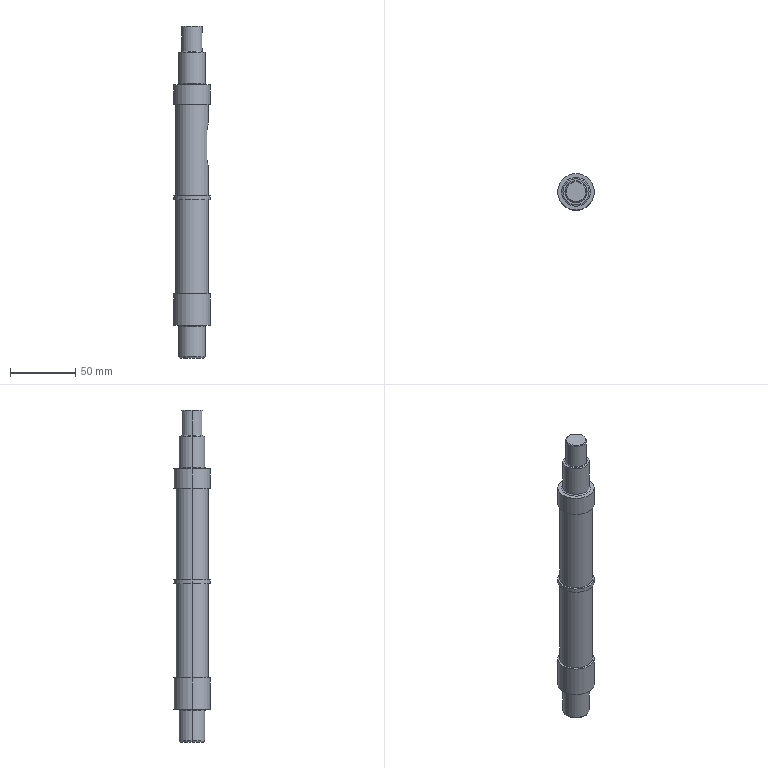Part | SolidWorks | features ICE 6, Fillet 3, Chamfer 2, Revolution 1 | 1 solid | 47 faces | box 28 x 28 x 254.001 mm | volume 113711 mm3 | cylinder 21 | plane 14 | torus 6 | cone 4 | spline 2 | commonest cylinder face diameters 28 x6 16 x4 20 x4 25 x4 10 x3
STEP:
#1=CARTESIAN_POINT('',(7.5,0.,-107.));
#2=VERTEX_POINT('',#1);
#3=CARTESIAN_POINT('',(7.5,5.,-102.));
#4=VERTEX_POINT('',#3);
#5=CARTESIAN_POINT('',(7.5,0.,-102.));
#6=DIRECTION('',(1.,0.,0.));
#7=DIRECTION('',(0.,0.,-1.));
#8=AXIS2_PLACEMENT_3D('',#5,#6,#7);
#9=CIRCLE('',#8,5.);
#10=EDGE_CURVE('',#2,#4,#9,.T.);
#11=ORIENTED_EDGE('',*,*,#10,.F.);
#12=CARTESIAN_POINT('',(12.5,0.,-107.));
#13=VERTEX_POINT('',#12);
#14=CARTESIAN_POINT('',(7.5,0.,-107.));
#15=DIRECTION('',(1.,0.,0.));
#16=VECTOR('',#15,1000.);
#17=LINE('',#14,#16);
#18=EDGE_CURVE('',#2,#13,#17,.T.);
#19=ORIENTED_EDGE('',*,*,#18,.T.);
#20=CARTESIAN_POINT('',(11.456,5.,-102.));
#21=VERTEX_POINT('',#20);
#22=CARTESIAN_POINT('',(11.456,5.,-102.));
#23=CARTESIAN_POINT('',(11.456,5.,-102.334));
#24=CARTESIAN_POINT('',(11.471,4.967,-102.662));
#25=CARTESIAN_POINT('',(11.526,4.838,-103.306));
#26=CARTESIAN_POINT('',(11.567,4.74,-103.625));
#27=CARTESIAN_POINT('',(11.667,4.488,-104.229));
#28=CARTESIAN_POINT('',(11.726,4.334,-104.515));
#29=CARTESIAN_POINT('',(11.854,3.971,-105.056));
#30=CARTESIAN_POINT('',(11.923,3.763,-105.309));
#31=CARTESIAN_POINT('',(12.057,3.306,-105.765));
#32=CARTESIAN_POINT('',(12.124,3.055,-105.971));
#33=CARTESIAN_POINT('',(12.248,2.511,-106.336));
#34=CARTESIAN_POINT('',(12.304,2.225,-106.489));
#35=CARTESIAN_POINT('',(12.374,1.774,-106.677));
#36=CARTESIAN_POINT('',(12.396,1.621,-106.733));
#37=CARTESIAN_POINT('',(12.433,1.305,-106.829));
#38=CARTESIAN_POINT('',(12.449,1.143,-106.87));
#39=CARTESIAN_POINT('',(12.487,0.6575,-106.968));
#40=CARTESIAN_POINT('',(12.5,0.3304,-107.));
#41=CARTESIAN_POINT('',(12.5,0.,-107.));
#42=B_SPLINE_CURVE_WITH_KNOTS('',3,(#22,#23,#24,#25,#26,#27,#28,#29,#30,#31,#32,#33,#34,#35,#36,#37,#38,#39,#40,#41),.UNSPECIFIED.,.F.,.F.,(4,2,2,2,2,2,2,2,2,4),(0.,0.0009877,0.001975,0.002963,0.003951,0.004939,0.005926,0.00642,0.006914,0.007902),.UNSPECIFIED.);
#43=EDGE_CURVE('',#21,#13,#42,.T.);
#44=ORIENTED_EDGE('',*,*,#43,.F.);
#45=CARTESIAN_POINT('',(7.5,5.,-102.));
#46=DIRECTION('',(1.,0.,0.));
#47=VECTOR('',#46,1000.);
#48=LINE('',#45,#47);
#49=EDGE_CURVE('',#4,#21,#48,.T.);
#50=ORIENTED_EDGE('',*,*,#49,.F.);
#51=EDGE_LOOP('',(#11,#19,#44,#50));
#52=FACE_OUTER_BOUND('',#51,.T.);
#53=CARTESIAN_POINT('',(7.5,0.,-102.));
#54=DIRECTION('',(1.,0.,0.));
#55=DIRECTION('',(0.,0.,-1.));
#56=AXIS2_PLACEMENT_3D('',#53,#54,#55);
#57=CYLINDRICAL_SURFACE('',#56,5.);
#58=ADVANCED_FACE('',(#52),#57,.F.);
#59=CARTESIAN_POINT('',(-12.5,0.,-130.));
#60=VERTEX_POINT('',#59);
#61=CARTESIAN_POINT('',(12.5,0.,-130.));
#62=VERTEX_POINT('',#61);
#63=CARTESIAN_POINT('',(0.,0.,-130.));
#64=DIRECTION('',(0.,0.,-1.));
#65=DIRECTION('',(-1.,0.,0.));
#66=AXIS2_PLACEMENT_3D('',#63,#64,#65);
#67=CIRCLE('',#66,12.5);
#68=EDGE_CURVE('',#60,#62,#67,.T.);
#69=ORIENTED_EDGE('',*,*,#68,.F.);
#70=CARTESIAN_POINT('',(-12.5,0.,-60.));
#71=VERTEX_POINT('',#70);
#72=CARTESIAN_POINT('',(-12.5,0.,0.));
#73=DIRECTION('',(0.,0.,1.));
#74=VECTOR('',#73,1000.);
#75=LINE('',#72,#74);
#76=EDGE_CURVE('',#60,#71,#75,.T.);
#77=ORIENTED_EDGE('',*,*,#76,.T.);
#78=CARTESIAN_POINT('',(12.5,0.,-60.));
#79=VERTEX_POINT('',#78);
#80=CARTESIAN_POINT('',(0.,0.,-60.));
#81=DIRECTION('',(0.,0.,1.));
#82=DIRECTION('',(1.,0.,0.));
#83=AXIS2_PLACEMENT_3D('',#80,#81,#82);
#84=CIRCLE('',#83,12.5);
#85=EDGE_CURVE('',#79,#71,#84,.T.);
#86=ORIENTED_EDGE('',*,*,#85,.F.);
#87=CARTESIAN_POINT('',(12.5,0.,-75.));
#88=VERTEX_POINT('',#87);
#89=CARTESIAN_POINT('',(12.5,0.,0.));
#90=DIRECTION('',(0.,0.,1.));
#91=VECTOR('',#90,1000.);
#92=LINE('',#89,#91);
#93=EDGE_CURVE('',#88,#79,#92,.T.);
#94=ORIENTED_EDGE('',*,*,#93,.F.);
#95=CARTESIAN_POINT('',(11.456,5.,-80.));
#96=VERTEX_POINT('',#95);
#97=CARTESIAN_POINT('',(12.5,0.,-75.));
#98=CARTESIAN_POINT('',(12.5,0.3299,-75.));
#99=CARTESIAN_POINT('',(12.487,0.6645,-75.033));
#100=CARTESIAN_POINT('',(12.436,1.308,-75.163));
#101=CARTESIAN_POINT('',(12.398,1.622,-75.259));
#102=CARTESIAN_POINT('',(12.303,2.231,-75.513));
#103=CARTESIAN_POINT('',(12.247,2.517,-75.668));
#104=CARTESIAN_POINT('',(12.124,3.055,-76.029));
#105=CARTESIAN_POINT('',(12.056,3.309,-76.238));
#106=CARTESIAN_POINT('',(11.922,3.766,-76.695));
#107=CARTESIAN_POINT('',(11.854,3.97,-76.944));
#108=CARTESIAN_POINT('',(11.727,4.332,-77.483));
#109=CARTESIAN_POINT('',(11.667,4.489,-77.773));
#110=CARTESIAN_POINT('',(11.568,4.739,-78.373));
#111=CARTESIAN_POINT('',(11.527,4.835,-78.684));
#112=CARTESIAN_POINT('',(11.471,4.967,-79.334));
#113=CARTESIAN_POINT('',(11.456,5.,-79.666));
#114=CARTESIAN_POINT('',(11.456,5.,-80.));
#115=B_SPLINE_CURVE_WITH_KNOTS('',3,(#97,#98,#99,#100,#101,#102,#103,#104,#105,#106,#107,#108,#109,#110,#111,#112,#113,#114),.UNSPECIFIED.,.F.,.F.,(4,2,2,2,2,2,2,2,4),(0.007902,0.008888,0.009874,0.01086,0.01185,0.01283,0.01382,0.01481,0.01579),.UNSPECIFIED.);
#116=EDGE_CURVE('',#88,#96,#115,.T.);
#117=ORIENTED_EDGE('',*,*,#116,.T.);
#118=CARTESIAN_POINT('',(11.456,5.,0.));
#119=DIRECTION('',(0.,0.,-1.));
#120=VECTOR('',#119,1000.);
#121=LINE('',#118,#120);
#122=EDGE_CURVE('',#96,#21,#121,.T.);
#123=ORIENTED_EDGE('',*,*,#122,.T.);
#124=ORIENTED_EDGE('',*,*,#43,.T.);
#125=CARTESIAN_POINT('',(12.5,0.,0.));
#126=DIRECTION('',(0.,0.,1.));
#127=VECTOR('',#126,1000.);
#128=LINE('',#125,#127);
#129=EDGE_CURVE('',#62,#13,#128,.T.);
#130=ORIENTED_EDGE('',*,*,#129,.F.);
#131=EDGE_LOOP('',(#69,#77,#86,#94,#117,#123,#124,#130));
#132=FACE_OUTER_BOUND('',#131,.T.);
#133=CARTESIAN_POINT('',(0.,0.,0.));
#134=DIRECTION('',(0.,0.,1.));
#135=DIRECTION('',(1.,0.,0.));
#136=AXIS2_PLACEMENT_3D('',#133,#134,#135);
#137=CYLINDRICAL_SURFACE('',#136,12.5);
#138=ADVANCED_FACE('',(#132),#137,.T.);
#139=CARTESIAN_POINT('',(14.,0.,-60.));
#140=VERTEX_POINT('',#139);
#141=CARTESIAN_POINT('',(-14.,0.,-60.));
#142=VERTEX_POINT('',#141);
#143=CARTESIAN_POINT('',(0.,0.,-60.));
#144=DIRECTION('',(0.,0.,1.));
#145=DIRECTION('',(1.,0.,0.));
#146=AXIS2_PLACEMENT_3D('',#143,#144,#145);
#147=CIRCLE('',#146,14.);
#148=EDGE_CURVE('',#140,#142,#147,.T.);
#149=ORIENTED_EDGE('',*,*,#148,.T.);
#150=CARTESIAN_POINT('',(-14.,0.,-45.));
#151=VERTEX_POINT('',#150);
#152=CARTESIAN_POINT('',(-14.,0.,0.));
#153=DIRECTION('',(0.,0.,1.));
#154=VECTOR('',#153,1000.);
#155=LINE('',#152,#154);
#156=EDGE_CURVE('',#142,#151,#155,.T.);
#157=ORIENTED_EDGE('',*,*,#156,.T.);
#158=CARTESIAN_POINT('',(14.,0.,-45.));
#159=VERTEX_POINT('',#158);
#160=CARTESIAN_POINT('',(0.,0.,-45.));
#161=DIRECTION('',(0.,0.,1.));
#162=DIRECTION('',(1.,0.,0.));
#163=AXIS2_PLACEMENT_3D('',#160,#161,#162);
#164=CIRCLE('',#163,14.);
#165=EDGE_CURVE('',#159,#151,#164,.T.);
#166=ORIENTED_EDGE('',*,*,#165,.F.);
#167=CARTESIAN_POINT('',(14.,0.,0.));
#168=DIRECTION('',(0.,0.,1.));
#169=VECTOR('',#168,1000.);
#170=LINE('',#167,#169);
#171=EDGE_CURVE('',#140,#159,#170,.T.);
#172=ORIENTED_EDGE('',*,*,#171,.F.);
#173=EDGE_LOOP('',(#149,#157,#166,#172));
#174=FACE_OUTER_BOUND('',#173,.T.);
#175=CARTESIAN_POINT('',(0.,0.,0.));
#176=DIRECTION('',(0.,0.,1.));
#177=DIRECTION('',(1.,0.,0.));
#178=AXIS2_PLACEMENT_3D('',#175,#176,#177);
#179=CYLINDRICAL_SURFACE('',#178,14.);
#180=ADVANCED_FACE('',(#174),#179,.T.);
#181=CARTESIAN_POINT('',(11.,0.,-45.));
#182=VERTEX_POINT('',#181);
#183=CARTESIAN_POINT('',(-11.,0.,-45.));
#184=VERTEX_POINT('',#183);
#185=CARTESIAN_POINT('',(0.,0.,-45.));
#186=DIRECTION('',(0.,0.,-1.));
#187=DIRECTION('',(-1.,0.,0.));
#188=AXIS2_PLACEMENT_3D('',#185,#186,#187);
#189=CIRCLE('',#188,11.);
#190=EDGE_CURVE('',#182,#184,#189,.T.);
#191=ORIENTED_EDGE('',*,*,#190,.F.);
#192=CARTESIAN_POINT('',(10.,0.,-44.));
#193=VERTEX_POINT('',#192);
#194=CARTESIAN_POINT('',(11.,0.,-44.));
#195=DIRECTION('',(0.,1.,0.));
#196=DIRECTION('',(-1.,0.,0.));
#197=AXIS2_PLACEMENT_3D('',#194,#195,#196);
#198=CIRCLE('',#197,1.);
#199=EDGE_CURVE('',#182,#193,#198,.T.);
#200=ORIENTED_EDGE('',*,*,#199,.T.);
#201=CARTESIAN_POINT('',(-10.,0.,-44.));
#202=VERTEX_POINT('',#201);
#203=CARTESIAN_POINT('',(0.,0.,-44.));
#204=DIRECTION('',(0.,0.,1.));
#205=DIRECTION('',(-1.,0.,0.));
#206=AXIS2_PLACEMENT_3D('',#203,#204,#205);
#207=CIRCLE('',#206,10.);
#208=EDGE_CURVE('',#202,#193,#207,.T.);
#209=ORIENTED_EDGE('',*,*,#208,.F.);
#210=CARTESIAN_POINT('',(-11.,0.,-44.));
#211=DIRECTION('',(0.,-1.,0.));
#212=DIRECTION('',(0.,0.,-1.));
#213=AXIS2_PLACEMENT_3D('',#210,#211,#212);
#214=CIRCLE('',#213,1.);
#215=EDGE_CURVE('',#184,#202,#214,.T.);
#216=ORIENTED_EDGE('',*,*,#215,.F.);
#217=EDGE_LOOP('',(#191,#200,#209,#216));
#218=FACE_OUTER_BOUND('',#217,.T.);
#219=CARTESIAN_POINT('',(0.,0.,-44.));
#220=DIRECTION('',(0.,0.,-1.));
#221=DIRECTION('',(-1.,0.,0.));
#222=AXIS2_PLACEMENT_3D('',#219,#220,#221);
#223=TOROIDAL_SURFACE('',#222,11.,1.);
#224=ADVANCED_FACE('',(#218),#223,.F.);
#225=CARTESIAN_POINT('',(0.,0.,-44.));
#226=DIRECTION('',(0.,0.,1.));
#227=DIRECTION('',(-1.,0.,0.));
#228=AXIS2_PLACEMENT_3D('',#225,#226,#227);
#229=CIRCLE('',#228,10.);
#230=EDGE_CURVE('',#193,#202,#229,.T.);
#231=ORIENTED_EDGE('',*,*,#230,.T.);
#232=CARTESIAN_POINT('',(-10.,0.,-20.));
#233=VERTEX_POINT('',#232);
#234=CARTESIAN_POINT('',(-10.,0.,0.));
#235=DIRECTION('',(0.,0.,1.));
#236=VECTOR('',#235,1000.);
#237=LINE('',#234,#236);
#238=EDGE_CURVE('',#202,#233,#237,.T.);
#239=ORIENTED_EDGE('',*,*,#238,.T.);
#240=CARTESIAN_POINT('',(10.,0.,-20.));
#241=VERTEX_POINT('',#240);
#242=CARTESIAN_POINT('',(0.,0.,-20.));
#243=DIRECTION('',(0.,0.,1.));
#244=DIRECTION('',(1.,0.,0.));
#245=AXIS2_PLACEMENT_3D('',#242,#243,#244);
#246=CIRCLE('',#245,10.);
#247=EDGE_CURVE('',#241,#233,#246,.T.);
#248=ORIENTED_EDGE('',*,*,#247,.F.);
#249=CARTESIAN_POINT('',(10.,0.,0.));
#250=DIRECTION('',(0.,0.,1.));
#251=VECTOR('',#250,1000.);
#252=LINE('',#249,#251);
#253=EDGE_CURVE('',#193,#241,#252,.T.);
#254=ORIENTED_EDGE('',*,*,#253,.F.);
#255=EDGE_LOOP('',(#231,#239,#248,#254));
#256=FACE_OUTER_BOUND('',#255,.T.);
#257=CARTESIAN_POINT('',(0.,0.,0.));
#258=DIRECTION('',(0.,0.,1.));
#259=DIRECTION('',(1.,0.,0.));
#260=AXIS2_PLACEMENT_3D('',#257,#258,#259);
#261=CYLINDRICAL_SURFACE('',#260,10.);
#262=ADVANCED_FACE('',(#256),#261,.T.);
#263=CARTESIAN_POINT('',(8.,0.,-19.5));
#264=VERTEX_POINT('',#263);
#265=CARTESIAN_POINT('',(-8.,0.,-19.5));
#266=VERTEX_POINT('',#265);
#267=CARTESIAN_POINT('',(0.,0.,-19.5));
#268=DIRECTION('',(0.,0.,1.));
#269=DIRECTION('',(-1.,0.,0.));
#270=AXIS2_PLACEMENT_3D('',#267,#268,#269);
#271=CIRCLE('',#270,8.);
#272=EDGE_CURVE('',#264,#266,#271,.T.);
#273=ORIENTED_EDGE('',*,*,#272,.F.);
#274=CARTESIAN_POINT('',(8.5,0.,-20.));
#275=VERTEX_POINT('',#274);
#276=CARTESIAN_POINT('',(8.,0.,-19.5));
#277=DIRECTION('',(0.7071,0.,-0.7071));
#278=VECTOR('',#277,1000.);
#279=LINE('',#276,#278);
#280=EDGE_CURVE('',#264,#275,#279,.T.);
#281=ORIENTED_EDGE('',*,*,#280,.T.);
#282=CARTESIAN_POINT('',(-8.5,0.,-20.));
#283=VERTEX_POINT('',#282);
#284=CARTESIAN_POINT('',(0.,0.,-20.));
#285=DIRECTION('',(0.,0.,-1.));
#286=DIRECTION('',(-1.,0.,0.));
#287=AXIS2_PLACEMENT_3D('',#284,#285,#286);
#288=CIRCLE('',#287,8.5);
#289=EDGE_CURVE('',#283,#275,#288,.T.);
#290=ORIENTED_EDGE('',*,*,#289,.F.);
#291=CARTESIAN_POINT('',(-8.,0.,-19.5));
#292=DIRECTION('',(-0.7071,0.,-0.7071));
#293=VECTOR('',#292,1000.);
#294=LINE('',#291,#293);
#295=EDGE_CURVE('',#266,#283,#294,.T.);
#296=ORIENTED_EDGE('',*,*,#295,.F.);
#297=EDGE_LOOP('',(#273,#281,#290,#296));
#298=FACE_OUTER_BOUND('',#297,.T.);
#299=CARTESIAN_POINT('',(0.,0.,-19.5));
#300=DIRECTION('',(0.,0.,-1.));
#301=DIRECTION('',(-1.,0.,0.));
#302=AXIS2_PLACEMENT_3D('',#299,#300,#301);
#303=CONICAL_SURFACE('',#302,8.,0.7854);
#304=ADVANCED_FACE('',(#298),#303,.T.);
#305=ORIENTED_EDGE('',*,*,#272,.T.);
#306=CARTESIAN_POINT('',(-8.,0.,-0.5));
#307=VERTEX_POINT('',#306);
#308=CARTESIAN_POINT('',(-8.,0.,0.));
#309=DIRECTION('',(0.,0.,1.));
#310=VECTOR('',#309,1000.);
#311=LINE('',#308,#310);
#312=EDGE_CURVE('',#266,#307,#311,.T.);
#313=ORIENTED_EDGE('',*,*,#312,.T.);
#314=CARTESIAN_POINT('',(8.,0.,-0.5));
#315=VERTEX_POINT('',#314);
#316=CARTESIAN_POINT('',(0.,0.,-0.5));
#317=DIRECTION('',(0.,0.,-1.));
#318=DIRECTION('',(-1.,0.,0.));
#319=AXIS2_PLACEMENT_3D('',#316,#317,#318);
#320=CIRCLE('',#319,8.);
#321=EDGE_CURVE('',#307,#315,#320,.T.);
#322=ORIENTED_EDGE('',*,*,#321,.T.);
#323=CARTESIAN_POINT('',(8.,0.000001723,-3.056));
#324=VERTEX_POINT('',#323);
#325=CARTESIAN_POINT('',(8.,0.,0.));
#326=DIRECTION('',(0.,0.,1.));
#327=VECTOR('',#326,1000.);
#328=LINE('',#325,#327);
#329=EDGE_CURVE('',#324,#315,#328,.T.);
#330=ORIENTED_EDGE('',*,*,#329,.F.);
#331=CARTESIAN_POINT('',(7.599,2.5,-5.556));
#332=VERTEX_POINT('',#331);
#333=CARTESIAN_POINT('',(7.599,2.5,-5.556));
#334=CARTESIAN_POINT('',(7.599,2.5,-4.891));
#335=CARTESIAN_POINT('',(7.698,2.226,-4.246));
#336=CARTESIAN_POINT('',(7.906,1.31,-3.33));
#337=CARTESIAN_POINT('',(8.,0.6593,-3.056));
#338=CARTESIAN_POINT('',(8.,0.00169,-3.056));
#339=CARTESIAN_POINT('',(8.,0.000846,-3.056));
#340=CARTESIAN_POINT('',(8.,0.000001723,-3.056));
#341=B_SPLINE_CURVE_WITH_KNOTS('',3,(#333,#334,#335,#336,#337,#338,#339,#340),.UNSPECIFIED.,.F.,.F.,(4,2,2,4),(0.,0.25,0.5,0.5003),.UNSPECIFIED.);
#342=EDGE_CURVE('',#332,#324,#341,.T.);
#343=ORIENTED_EDGE('',*,*,#342,.F.);
#344=CARTESIAN_POINT('',(7.599,2.5,-16.556));
#345=VERTEX_POINT('',#344);
#346=CARTESIAN_POINT('',(7.599,2.5,0.));
#347=DIRECTION('',(0.,0.,1.));
#348=VECTOR('',#347,1000.);
#349=LINE('',#346,#348);
#350=EDGE_CURVE('',#345,#332,#349,.T.);
#351=ORIENTED_EDGE('',*,*,#350,.F.);
#352=CARTESIAN_POINT('',(8.,-0.000001723,-19.056));
#353=VERTEX_POINT('',#352);
#354=CARTESIAN_POINT('',(8.,-0.000001723,-19.056));
#355=CARTESIAN_POINT('',(8.,0.6559,-19.056));
#356=CARTESIAN_POINT('',(7.907,1.307,-18.784));
#357=CARTESIAN_POINT('',(7.698,2.228,-17.863));
#358=CARTESIAN_POINT('',(7.599,2.5,-17.221));
#359=CARTESIAN_POINT('',(7.599,2.5,-16.556));
#360=B_SPLINE_CURVE_WITH_KNOTS('',3,(#354,#355,#356,#357,#358,#359),.UNSPECIFIED.,.F.,.F.,(4,2,4),(0.5003,0.75,1.),.UNSPECIFIED.);
#361=EDGE_CURVE('',#353,#345,#360,.T.);
#362=ORIENTED_EDGE('',*,*,#361,.F.);
#363=CARTESIAN_POINT('',(8.,0.,0.));
#364=DIRECTION('',(0.,0.,1.));
#365=VECTOR('',#364,1000.);
#366=LINE('',#363,#365);
#367=EDGE_CURVE('',#264,#353,#366,.T.);
#368=ORIENTED_EDGE('',*,*,#367,.F.);
#369=EDGE_LOOP('',(#305,#313,#322,#330,#343,#351,#362,#368));
#370=FACE_OUTER_BOUND('',#369,.T.);
#371=CARTESIAN_POINT('',(0.,0.,0.));
#372=DIRECTION('',(0.,0.,1.));
#373=DIRECTION('',(1.,0.,0.));
#374=AXIS2_PLACEMENT_3D('',#371,#372,#373);
#375=CYLINDRICAL_SURFACE('',#374,8.);
#376=ADVANCED_FACE('',(#370),#375,.T.);
#377=CARTESIAN_POINT('',(7.5,0.,0.));
#378=VERTEX_POINT('',#377);
#379=CARTESIAN_POINT('',(-7.5,0.,0.));
#380=VERTEX_POINT('',#379);
#381=CARTESIAN_POINT('',(0.,0.,0.));
#382=DIRECTION('',(0.,0.,1.));
#383=DIRECTION('',(-1.,0.,0.));
#384=AXIS2_PLACEMENT_3D('',#381,#382,#383);
#385=CIRCLE('',#384,7.5);
#386=EDGE_CURVE('',#378,#380,#385,.T.);
#387=ORIENTED_EDGE('',*,*,#386,.F.);
#388=CARTESIAN_POINT('',(7.5,0.,0.));
#389=DIRECTION('',(0.7071,0.,-0.7071));
#390=VECTOR('',#389,1000.);
#391=LINE('',#388,#390);
#392=EDGE_CURVE('',#378,#315,#391,.T.);
#393=ORIENTED_EDGE('',*,*,#392,.T.);
#394=ORIENTED_EDGE('',*,*,#321,.F.);
#395=CARTESIAN_POINT('',(-7.5,0.,0.));
#396=DIRECTION('',(-0.7071,0.,-0.7071));
#397=VECTOR('',#396,1000.);
#398=LINE('',#395,#397);
#399=EDGE_CURVE('',#380,#307,#398,.T.);
#400=ORIENTED_EDGE('',*,*,#399,.F.);
#401=EDGE_LOOP('',(#387,#393,#394,#400));
#402=FACE_OUTER_BOUND('',#401,.T.);
#403=CARTESIAN_POINT('',(0.,0.,0.));
#404=DIRECTION('',(0.,0.,-1.));
#405=DIRECTION('',(-1.,0.,0.));
#406=AXIS2_PLACEMENT_3D('',#403,#404,#405);
#407=CONICAL_SURFACE('',#406,7.5,0.7854);
#408=ADVANCED_FACE('',(#402),#407,.T.);
#409=CARTESIAN_POINT('',(4.899,-2.5,-16.556));
#410=VERTEX_POINT('',#409);
#411=CARTESIAN_POINT('',(5.3,0.000000481,-19.056));
#412=VERTEX_POINT('',#411);
#413=CARTESIAN_POINT('',(4.899,-2.5,-16.556));
#414=CARTESIAN_POINT('',(4.899,-2.5,-16.887));
#415=CARTESIAN_POINT('',(4.923,-2.431,-17.217));
#416=CARTESIAN_POINT('',(4.999,-2.179,-17.819));
#417=CARTESIAN_POINT('',(5.051,-1.995,-18.096));
#418=CARTESIAN_POINT('',(5.154,-1.539,-18.552));
#419=CARTESIAN_POINT('',(5.206,-1.261,-18.736));
#420=CARTESIAN_POINT('',(5.279,-0.6553,-18.988));
#421=CARTESIAN_POINT('',(5.3,-0.3268,-19.056));
#422=CARTESIAN_POINT('',(5.3,0.000000481,-19.056));
#423=B_SPLINE_CURVE_WITH_KNOTS('',3,(#413,#414,#415,#416,#417,#418,#419,#420,#421,#422),.UNSPECIFIED.,.F.,.F.,(4,2,2,2,4),(0.,0.1251,0.2502,0.3752,0.5003),.UNSPECIFIED.);
#424=EDGE_CURVE('',#410,#412,#423,.T.);
#425=ORIENTED_EDGE('',*,*,#424,.T.);
#426=CARTESIAN_POINT('',(5.3,-0.000000481,-3.056));
#427=VERTEX_POINT('',#426);
#428=CARTESIAN_POINT('',(5.3,0.,0.));
#429=DIRECTION('',(0.,0.,1.));
#430=VECTOR('',#429,1000.);
#431=LINE('',#428,#430);
#432=EDGE_CURVE('',#412,#427,#431,.T.);
#433=ORIENTED_EDGE('',*,*,#432,.T.);
#434=CARTESIAN_POINT('',(4.899,-2.5,-5.556));
#435=VERTEX_POINT('',#434);
#436=CARTESIAN_POINT('',(5.3,-0.000000481,-3.056));
#437=CARTESIAN_POINT('',(5.3,-0.3264,-3.056));
#438=CARTESIAN_POINT('',(5.279,-0.655,-3.124));
#439=CARTESIAN_POINT('',(5.206,-1.26,-3.375));
#440=CARTESIAN_POINT('',(5.154,-1.538,-3.559));
#441=CARTESIAN_POINT('',(5.05,-1.998,-4.018));
#442=CARTESIAN_POINT('',(4.998,-2.181,-4.293));
#443=CARTESIAN_POINT('',(4.922,-2.432,-4.898));
#444=CARTESIAN_POINT('',(4.899,-2.5,-5.225));
#445=CARTESIAN_POINT('',(4.899,-2.5,-5.556));
#446=B_SPLINE_CURVE_WITH_KNOTS('',3,(#436,#437,#438,#439,#440,#441,#442,#443,#444,#445),.UNSPECIFIED.,.F.,.F.,(4,2,2,2,4),(0.5003,0.6252,0.7502,0.8751,1.),.UNSPECIFIED.);
#447=EDGE_CURVE('',#427,#435,#446,.T.);
#448=ORIENTED_EDGE('',*,*,#447,.T.);
#449=CARTESIAN_POINT('',(4.899,-2.5,0.));
#450=DIRECTION('',(0.,0.,1.));
#451=VECTOR('',#450,1000.);
#452=LINE('',#449,#451);
#453=EDGE_CURVE('',#410,#435,#452,.T.);
#454=ORIENTED_EDGE('',*,*,#453,.F.);
#455=EDGE_LOOP('',(#425,#433,#448,#454));
#456=FACE_OUTER_BOUND('',#455,.T.);
#457=CARTESIAN_POINT('',(-2.7,0.,0.));
#458=DIRECTION('',(0.,0.,1.));
#459=DIRECTION('',(1.,0.,0.));
#460=AXIS2_PLACEMENT_3D('',#457,#458,#459);
#461=CYLINDRICAL_SURFACE('',#460,8.);
#462=ADVANCED_FACE('',(#456),#461,.T.);
#463=CARTESIAN_POINT('',(-11.,0.,-229.));
#464=VERTEX_POINT('',#463);
#465=CARTESIAN_POINT('',(11.,0.,-229.));
#466=VERTEX_POINT('',#465);
#467=CARTESIAN_POINT('',(0.,0.,-229.));
#468=DIRECTION('',(0.,0.,1.));
#469=DIRECTION('',(1.,0.,0.));
#470=AXIS2_PLACEMENT_3D('',#467,#468,#469);
#471=CIRCLE('',#470,11.);
#472=EDGE_CURVE('',#464,#466,#471,.T.);
#473=ORIENTED_EDGE('',*,*,#472,.F.);
#474=CARTESIAN_POINT('',(-10.,0.,-230.));
#475=VERTEX_POINT('',#474);
#476=CARTESIAN_POINT('',(-11.,0.,-230.));
#477=DIRECTION('',(0.,1.,0.));
#478=DIRECTION('',(-1.,0.,0.));
#479=AXIS2_PLACEMENT_3D('',#476,#477,#478);
#480=CIRCLE('',#479,1.);
#481=EDGE_CURVE('',#464,#475,#480,.T.);
#482=ORIENTED_EDGE('',*,*,#481,.T.);
#483=CARTESIAN_POINT('',(10.,0.,-230.));
#484=VERTEX_POINT('',#483);
#485=CARTESIAN_POINT('',(0.,0.,-230.));
#486=DIRECTION('',(0.,0.,-1.));
#487=DIRECTION('',(1.,0.,0.));
#488=AXIS2_PLACEMENT_3D('',#485,#486,#487);
#489=CIRCLE('',#488,10.);
#490=EDGE_CURVE('',#484,#475,#489,.T.);
#491=ORIENTED_EDGE('',*,*,#490,.F.);
#492=CARTESIAN_POINT('',(11.,0.,-230.));
#493=DIRECTION('',(0.,-1.,0.));
#494=DIRECTION('',(0.,0.,-1.));
#495=AXIS2_PLACEMENT_3D('',#492,#493,#494);
#496=CIRCLE('',#495,1.);
#497=EDGE_CURVE('',#466,#484,#496,.T.);
#498=ORIENTED_EDGE('',*,*,#497,.F.);
#499=EDGE_LOOP('',(#473,#482,#491,#498));
#500=FACE_OUTER_BOUND('',#499,.T.);
#501=CARTESIAN_POINT('',(0.,0.,-230.));
#502=DIRECTION('',(0.,0.,1.));
#503=DIRECTION('',(1.,0.,0.));
#504=AXIS2_PLACEMENT_3D('',#501,#502,#503);
#505=TOROIDAL_SURFACE('',#504,11.,1.);
#506=ADVANCED_FACE('',(#500),#505,.F.);
#507=CARTESIAN_POINT('',(12.5,0.,-205.));
#508=VERTEX_POINT('',#507);
#509=CARTESIAN_POINT('',(-12.5,0.,-205.));
#510=VERTEX_POINT('',#509);
#511=CARTESIAN_POINT('',(0.,0.,-205.));
#512=DIRECTION('',(0.,0.,1.));
#513=DIRECTION('',(1.,0.,0.));
#514=AXIS2_PLACEMENT_3D('',#511,#512,#513);
#515=CIRCLE('',#514,12.5);
#516=EDGE_CURVE('',#508,#510,#515,.T.);
#517=ORIENTED_EDGE('',*,*,#516,.T.);
#518=CARTESIAN_POINT('',(-12.5,0.,-133.));
#519=VERTEX_POINT('',#518);
#520=CARTESIAN_POINT('',(-12.5,0.,0.));
#521=DIRECTION('',(0.,0.,1.));
#522=VECTOR('',#521,1000.);
#523=LINE('',#520,#522);
#524=EDGE_CURVE('',#510,#519,#523,.T.);
#525=ORIENTED_EDGE('',*,*,#524,.T.);
#526=CARTESIAN_POINT('',(12.5,0.,-133.));
#527=VERTEX_POINT('',#526);
#528=CARTESIAN_POINT('',(0.,0.,-133.));
#529=DIRECTION('',(0.,0.,-1.));
#530=DIRECTION('',(-1.,0.,0.));
#531=AXIS2_PLACEMENT_3D('',#528,#529,#530);
#532=CIRCLE('',#531,12.5);
#533=EDGE_CURVE('',#519,#527,#532,.T.);
#534=ORIENTED_EDGE('',*,*,#533,.T.);
#535=CARTESIAN_POINT('',(12.5,0.,0.));
#536=DIRECTION('',(0.,0.,1.));
#537=VECTOR('',#536,1000.);
#538=LINE('',#535,#537);
#539=EDGE_CURVE('',#508,#527,#538,.T.);
#540=ORIENTED_EDGE('',*,*,#539,.F.);
#541=EDGE_LOOP('',(#517,#525,#534,#540));
#542=FACE_OUTER_BOUND('',#541,.T.);
#543=CARTESIAN_POINT('',(0.,0.,0.));
#544=DIRECTION('',(0.,0.,1.));
#545=DIRECTION('',(1.,0.,0.));
#546=AXIS2_PLACEMENT_3D('',#543,#544,#545);
#547=CYLINDRICAL_SURFACE('',#546,12.5);
#548=ADVANCED_FACE('',(#542),#547,.T.);
#549=CARTESIAN_POINT('',(14.,0.,-229.));
#550=VERTEX_POINT('',#549);
#551=CARTESIAN_POINT('',(-14.,0.,-229.));
#552=VERTEX_POINT('',#551);
#553=CARTESIAN_POINT('',(0.,0.,-229.));
#554=DIRECTION('',(0.,0.,1.));
#555=DIRECTION('',(1.,0.,0.));
#556=AXIS2_PLACEMENT_3D('',#553,#554,#555);
#557=CIRCLE('',#556,14.);
#558=EDGE_CURVE('',#550,#552,#557,.T.);
#559=ORIENTED_EDGE('',*,*,#558,.T.);
#560=CARTESIAN_POINT('',(-14.,0.,-205.));
#561=VERTEX_POINT('',#560);
#562=CARTESIAN_POINT('',(-14.,0.,0.));
#563=DIRECTION('',(0.,0.,1.));
#564=VECTOR('',#563,1000.);
#565=LINE('',#562,#564);
#566=EDGE_CURVE('',#552,#561,#565,.T.);
#567=ORIENTED_EDGE('',*,*,#566,.T.);
#568=CARTESIAN_POINT('',(14.,0.,-205.));
#569=VERTEX_POINT('',#568);
#570=CARTESIAN_POINT('',(0.,0.,-205.));
#571=DIRECTION('',(0.,0.,1.));
#572=DIRECTION('',(1.,0.,0.));
#573=AXIS2_PLACEMENT_3D('',#570,#571,#572);
#574=CIRCLE('',#573,14.);
#575=EDGE_CURVE('',#569,#561,#574,.T.);
#576=ORIENTED_EDGE('',*,*,#575,.F.);
#577=CARTESIAN_POINT('',(14.,0.,0.));
#578=DIRECTION('',(0.,0.,1.));
#579=VECTOR('',#578,1000.);
#580=LINE('',#577,#579);
#581=EDGE_CURVE('',#550,#569,#580,.T.);
#582=ORIENTED_EDGE('',*,*,#581,.F.);
#583=EDGE_LOOP('',(#559,#567,#576,#582));
#584=FACE_OUTER_BOUND('',#583,.T.);
#585=CARTESIAN_POINT('',(0.,0.,0.));
#586=DIRECTION('',(0.,0.,1.));
#587=DIRECTION('',(1.,0.,0.));
#588=AXIS2_PLACEMENT_3D('',#585,#586,#587);
#589=CYLINDRICAL_SURFACE('',#588,14.);
#590=ADVANCED_FACE('',(#584),#589,.T.);
#591=CARTESIAN_POINT('',(10.,0.,-253.001));
#592=VERTEX_POINT('',#591);
#593=CARTESIAN_POINT('',(-10.,0.,-253.001));
#594=VERTEX_POINT('',#593);
#595=CARTESIAN_POINT('',(0.,0.,-253.001));
#596=DIRECTION('',(0.,0.,1.));
#597=DIRECTION('',(-1.,0.,0.));
#598=AXIS2_PLACEMENT_3D('',#595,#596,#597);
#599=CIRCLE('',#598,10.);
#600=EDGE_CURVE('',#592,#594,#599,.T.);
#601=ORIENTED_EDGE('',*,*,#600,.T.);
#602=CARTESIAN_POINT('',(-10.,0.,0.));
#603=DIRECTION('',(0.,0.,1.));
#604=VECTOR('',#603,1000.);
#605=LINE('',#602,#604);
#606=EDGE_CURVE('',#594,#475,#605,.T.);
#607=ORIENTED_EDGE('',*,*,#606,.T.);
#608=CARTESIAN_POINT('',(0.,0.,-230.));
#609=DIRECTION('',(0.,0.,-1.));
#610=DIRECTION('',(1.,0.,0.));
#611=AXIS2_PLACEMENT_3D('',#608,#609,#610);
#612=CIRCLE('',#611,10.);
#613=EDGE_CURVE('',#475,#484,#612,.T.);
#614=ORIENTED_EDGE('',*,*,#613,.T.);
#615=CARTESIAN_POINT('',(10.,0.,0.));
#616=DIRECTION('',(0.,0.,1.));
#617=VECTOR('',#616,1000.);
#618=LINE('',#615,#617);
#619=EDGE_CURVE('',#592,#484,#618,.T.);
#620=ORIENTED_EDGE('',*,*,#619,.F.);
#621=EDGE_LOOP('',(#601,#607,#614,#620));
#622=FACE_OUTER_BOUND('',#621,.T.);
#623=CARTESIAN_POINT('',(0.,0.,0.));
#624=DIRECTION('',(0.,0.,1.));
#625=DIRECTION('',(1.,0.,0.));
#626=AXIS2_PLACEMENT_3D('',#623,#624,#625);
#627=CYLINDRICAL_SURFACE('',#626,10.);
#628=ADVANCED_FACE('',(#622),#627,.T.);
#629=ORIENTED_EDGE('',*,*,#600,.F.);
#630=CARTESIAN_POINT('',(9.,0.,-254.001));
#631=VERTEX_POINT('',#630);
#632=CARTESIAN_POINT('',(9.,0.,-253.001));
#633=DIRECTION('',(0.,1.,0.));
#634=DIRECTION('',(-1.,0.,0.));
#635=AXIS2_PLACEMENT_3D('',#632,#633,#634);
#636=CIRCLE('',#635,1.);
#637=EDGE_CURVE('',#592,#631,#636,.T.);
#638=ORIENTED_EDGE('',*,*,#637,.T.);
#639=CARTESIAN_POINT('',(-9.,0.,-254.001));
#640=VERTEX_POINT('',#639);
#641=CARTESIAN_POINT('',(0.,0.,-254.001));
#642=DIRECTION('',(0.,0.,-1.));
#643=DIRECTION('',(-1.,0.,0.));
#644=AXIS2_PLACEMENT_3D('',#641,#642,#643);
#645=CIRCLE('',#644,9.);
#646=EDGE_CURVE('',#640,#631,#645,.T.);
#647=ORIENTED_EDGE('',*,*,#646,.F.);
#648=CARTESIAN_POINT('',(-9.,0.,-253.001));
#649=DIRECTION('',(0.,-1.,0.));
#650=DIRECTION('',(0.,0.,-1.));
#651=AXIS2_PLACEMENT_3D('',#648,#649,#650);
#652=CIRCLE('',#651,1.);
#653=EDGE_CURVE('',#594,#640,#652,.T.);
#654=ORIENTED_EDGE('',*,*,#653,.F.);
#655=EDGE_LOOP('',(#629,#638,#647,#654));
#656=FACE_OUTER_BOUND('',#655,.T.);
#657=CARTESIAN_POINT('',(0.,0.,-253.001));
#658=DIRECTION('',(0.,0.,-1.));
#659=DIRECTION('',(-1.,0.,0.));
#660=AXIS2_PLACEMENT_3D('',#657,#658,#659);
#661=TOROIDAL_SURFACE('',#660,9.,1.);
#662=ADVANCED_FACE('',(#656),#661,.T.);
#663=CARTESIAN_POINT('',(-14.,0.,-130.));
#664=VERTEX_POINT('',#663);
#665=CARTESIAN_POINT('',(14.,0.,-130.));
#666=VERTEX_POINT('',#665);
#667=CARTESIAN_POINT('',(0.,0.,-130.));
#668=DIRECTION('',(0.,0.,-1.));
#669=DIRECTION('',(-1.,0.,0.));
#670=AXIS2_PLACEMENT_3D('',#667,#668,#669);
#671=CIRCLE('',#670,14.);
#672=EDGE_CURVE('',#664,#666,#671,.T.);
#673=ORIENTED_EDGE('',*,*,#672,.T.);
#674=CARTESIAN_POINT('',(14.,0.,-133.));
#675=VERTEX_POINT('',#674);
#676=CARTESIAN_POINT('',(14.,0.,-130.));
#677=DIRECTION('',(0.,0.,-1.));
#678=VECTOR('',#677,1000.);
#679=LINE('',#676,#678);
#680=EDGE_CURVE('',#666,#675,#679,.T.);
#681=ORIENTED_EDGE('',*,*,#680,.T.);
#682=CARTESIAN_POINT('',(-14.,0.,-133.));
#683=VERTEX_POINT('',#682);
#684=CARTESIAN_POINT('',(0.,0.,-133.));
#685=DIRECTION('',(0.,0.,-1.));
#686=DIRECTION('',(-1.,0.,0.));
#687=AXIS2_PLACEMENT_3D('',#684,#685,#686);
#688=CIRCLE('',#687,14.);
#689=EDGE_CURVE('',#683,#675,#688,.T.);
#690=ORIENTED_EDGE('',*,*,#689,.F.);
#691=CARTESIAN_POINT('',(-14.,0.,-130.));
#692=DIRECTION('',(0.,0.,-1.));
#693=VECTOR('',#692,1000.);
#694=LINE('',#691,#693);
#695=EDGE_CURVE('',#664,#683,#694,.T.);
#696=ORIENTED_EDGE('',*,*,#695,.F.);
#697=EDGE_LOOP('',(#673,#681,#690,#696));
#698=FACE_OUTER_BOUND('',#697,.T.);
#699=CARTESIAN_POINT('',(0.,0.,-130.));
#700=DIRECTION('',(0.,0.,-1.));
#701=DIRECTION('',(-1.,0.,0.));
#702=AXIS2_PLACEMENT_3D('',#699,#700,#701);
#703=CYLINDRICAL_SURFACE('',#702,14.);
#704=ADVANCED_FACE('',(#698),#703,.T.);
#705=ORIENTED_EDGE('',*,*,#680,.F.);
#706=CARTESIAN_POINT('',(0.,0.,-130.));
#707=DIRECTION('',(0.,0.,-1.));
#708=DIRECTION('',(-1.,0.,0.));
#709=AXIS2_PLACEMENT_3D('',#706,#707,#708);
#710=CIRCLE('',#709,14.);
#711=EDGE_CURVE('',#666,#664,#710,.T.);
#712=ORIENTED_EDGE('',*,*,#711,.T.);
#713=ORIENTED_EDGE('',*,*,#695,.T.);
#714=CARTESIAN_POINT('',(0.,0.,-133.));
#715=DIRECTION('',(0.,0.,-1.));
#716=DIRECTION('',(-1.,0.,0.));
#717=AXIS2_PLACEMENT_3D('',#714,#715,#716);
#718=CIRCLE('',#717,14.);
#719=EDGE_CURVE('',#675,#683,#718,.T.);
#720=ORIENTED_EDGE('',*,*,#719,.F.);
#721=EDGE_LOOP('',(#705,#712,#713,#720));
#722=FACE_OUTER_BOUND('',#721,.T.);
#723=CARTESIAN_POINT('',(0.,0.,-130.));
#724=DIRECTION('',(0.,0.,-1.));
#725=DIRECTION('',(-1.,0.,0.));
#726=AXIS2_PLACEMENT_3D('',#723,#724,#725);
#727=CYLINDRICAL_SURFACE('',#726,14.);
#728=ADVANCED_FACE('',(#722),#727,.T.);
#729=CARTESIAN_POINT('',(0.,0.,-130.));
#730=DIRECTION('',(0.,0.,-1.));
#731=DIRECTION('',(-1.,0.,0.));
#732=AXIS2_PLACEMENT_3D('',#729,#730,#731);
#733=CIRCLE('',#732,12.5);
#734=EDGE_CURVE('',#62,#60,#733,.T.);
#735=ORIENTED_EDGE('',*,*,#734,.T.);
#736=ORIENTED_EDGE('',*,*,#68,.T.);
#737=EDGE_LOOP('',(#735,#736));
#738=FACE_BOUND('',#737,.T.);
#739=ORIENTED_EDGE('',*,*,#672,.F.);
#740=ORIENTED_EDGE('',*,*,#711,.F.);
#741=EDGE_LOOP('',(#739,#740));
#742=FACE_OUTER_BOUND('',#741,.T.);
#743=CARTESIAN_POINT('',(0.,0.,-130.));
#744=DIRECTION('',(0.,0.,-1.));
#745=DIRECTION('',(-1.,0.,0.));
#746=AXIS2_PLACEMENT_3D('',#743,#744,#745);
#747=PLANE('',#746);
#748=ADVANCED_FACE('',(#738,#742),#747,.F.);
#749=CARTESIAN_POINT('',(0.,0.,-133.));
#750=DIRECTION('',(0.,0.,-1.));
#751=DIRECTION('',(-1.,0.,0.));
#752=AXIS2_PLACEMENT_3D('',#749,#750,#751);
#753=CIRCLE('',#752,12.5);
#754=EDGE_CURVE('',#527,#519,#753,.T.);
#755=ORIENTED_EDGE('',*,*,#754,.F.);
#756=ORIENTED_EDGE('',*,*,#533,.F.);
#757=EDGE_LOOP('',(#755,#756));
#758=FACE_BOUND('',#757,.T.);
#759=ORIENTED_EDGE('',*,*,#689,.T.);
#760=ORIENTED_EDGE('',*,*,#719,.T.);
#761=EDGE_LOOP('',(#759,#760));
#762=FACE_OUTER_BOUND('',#761,.T.);
#763=CARTESIAN_POINT('',(0.,0.,-133.));
#764=DIRECTION('',(0.,0.,-1.));
#765=DIRECTION('',(-1.,0.,0.));
#766=AXIS2_PLACEMENT_3D('',#763,#764,#765);
#767=PLANE('',#766);
#768=ADVANCED_FACE('',(#758,#762),#767,.T.);
#769=ORIENTED_EDGE('',*,*,#646,.T.);
#770=CARTESIAN_POINT('',(0.,0.,-254.001));
#771=DIRECTION('',(0.,0.,-1.));
#772=DIRECTION('',(-1.,0.,0.));
#773=AXIS2_PLACEMENT_3D('',#770,#771,#772);
#774=CIRCLE('',#773,9.);
#775=EDGE_CURVE('',#631,#640,#774,.T.);
#776=ORIENTED_EDGE('',*,*,#775,.T.);
#777=EDGE_LOOP('',(#769,#776));
#778=FACE_OUTER_BOUND('',#777,.T.);
#779=CARTESIAN_POINT('',(0.,0.,-254.001));
#780=DIRECTION('',(0.,0.,-1.));
#781=DIRECTION('',(-1.,0.,0.));
#782=AXIS2_PLACEMENT_3D('',#779,#780,#781);
#783=PLANE('',#782);
#784=ADVANCED_FACE('',(#778),#783,.T.);
#785=ORIENTED_EDGE('',*,*,#637,.F.);
#786=CARTESIAN_POINT('',(0.,0.,-253.001));
#787=DIRECTION('',(0.,0.,1.));
#788=DIRECTION('',(-1.,0.,0.));
#789=AXIS2_PLACEMENT_3D('',#786,#787,#788);
#790=CIRCLE('',#789,10.);
#791=EDGE_CURVE('',#594,#592,#790,.T.);
#792=ORIENTED_EDGE('',*,*,#791,.F.);
#793=ORIENTED_EDGE('',*,*,#653,.T.);
#794=ORIENTED_EDGE('',*,*,#775,.F.);
#795=EDGE_LOOP('',(#785,#792,#793,#794));
#796=FACE_OUTER_BOUND('',#795,.T.);
#797=CARTESIAN_POINT('',(0.,0.,-253.001));
#798=DIRECTION('',(0.,0.,-1.));
#799=DIRECTION('',(-1.,0.,0.));
#800=AXIS2_PLACEMENT_3D('',#797,#798,#799);
#801=TOROIDAL_SURFACE('',#800,9.,1.);
#802=ADVANCED_FACE('',(#796),#801,.T.);
#803=ORIENTED_EDGE('',*,*,#606,.F.);
#804=ORIENTED_EDGE('',*,*,#791,.T.);
#805=ORIENTED_EDGE('',*,*,#619,.T.);
#806=ORIENTED_EDGE('',*,*,#490,.T.);
#807=EDGE_LOOP('',(#803,#804,#805,#806));
#808=FACE_OUTER_BOUND('',#807,.T.);
#809=CARTESIAN_POINT('',(0.,0.,0.));
#810=DIRECTION('',(0.,0.,1.));
#811=DIRECTION('',(1.,0.,0.));
#812=AXIS2_PLACEMENT_3D('',#809,#810,#811);
#813=CYLINDRICAL_SURFACE('',#812,10.);
#814=ADVANCED_FACE('',(#808),#813,.T.);
#815=CARTESIAN_POINT('',(0.,0.,-229.));
#816=DIRECTION('',(0.,0.,1.));
#817=DIRECTION('',(1.,0.,0.));
#818=AXIS2_PLACEMENT_3D('',#815,#816,#817);
#819=CIRCLE('',#818,11.);
#820=EDGE_CURVE('',#466,#464,#819,.T.);
#821=ORIENTED_EDGE('',*,*,#820,.T.);
#822=ORIENTED_EDGE('',*,*,#472,.T.);
#823=EDGE_LOOP('',(#821,#822));
#824=FACE_BOUND('',#823,.T.);
#825=ORIENTED_EDGE('',*,*,#558,.F.);
#826=CARTESIAN_POINT('',(0.,0.,-229.));
#827=DIRECTION('',(0.,0.,1.));
#828=DIRECTION('',(1.,0.,0.));
#829=AXIS2_PLACEMENT_3D('',#826,#827,#828);
#830=CIRCLE('',#829,14.);
#831=EDGE_CURVE('',#552,#550,#830,.T.);
#832=ORIENTED_EDGE('',*,*,#831,.F.);
#833=EDGE_LOOP('',(#825,#832));
#834=FACE_OUTER_BOUND('',#833,.T.);
#835=CARTESIAN_POINT('',(0.,10.,-229.));
#836=DIRECTION('',(0.,0.,1.));
#837=DIRECTION('',(1.,0.,0.));
#838=AXIS2_PLACEMENT_3D('',#835,#836,#837);
#839=PLANE('',#838);
#840=ADVANCED_FACE('',(#824,#834),#839,.F.);
#841=ORIENTED_EDGE('',*,*,#566,.F.);
#842=ORIENTED_EDGE('',*,*,#831,.T.);
#843=ORIENTED_EDGE('',*,*,#581,.T.);
#844=CARTESIAN_POINT('',(0.,0.,-205.));
#845=DIRECTION('',(0.,0.,1.));
#846=DIRECTION('',(1.,0.,0.));
#847=AXIS2_PLACEMENT_3D('',#844,#845,#846);
#848=CIRCLE('',#847,14.);
#849=EDGE_CURVE('',#561,#569,#848,.T.);
#850=ORIENTED_EDGE('',*,*,#849,.F.);
#851=EDGE_LOOP('',(#841,#842,#843,#850));
#852=FACE_OUTER_BOUND('',#851,.T.);
#853=CARTESIAN_POINT('',(0.,0.,0.));
#854=DIRECTION('',(0.,0.,1.));
#855=DIRECTION('',(1.,0.,0.));
#856=AXIS2_PLACEMENT_3D('',#853,#854,#855);
#857=CYLINDRICAL_SURFACE('',#856,14.);
#858=ADVANCED_FACE('',(#852),#857,.T.);
#859=ORIENTED_EDGE('',*,*,#516,.F.);
#860=CARTESIAN_POINT('',(0.,0.,-205.));
#861=DIRECTION('',(0.,0.,1.));
#862=DIRECTION('',(1.,0.,0.));
#863=AXIS2_PLACEMENT_3D('',#860,#861,#862);
#864=CIRCLE('',#863,12.5);
#865=EDGE_CURVE('',#510,#508,#864,.T.);
#866=ORIENTED_EDGE('',*,*,#865,.F.);
#867=EDGE_LOOP('',(#859,#866));
#868=FACE_BOUND('',#867,.T.);
#869=ORIENTED_EDGE('',*,*,#575,.T.);
#870=ORIENTED_EDGE('',*,*,#849,.T.);
#871=EDGE_LOOP('',(#869,#870));
#872=FACE_OUTER_BOUND('',#871,.T.);
#873=CARTESIAN_POINT('',(0.,12.5,-205.));
#874=DIRECTION('',(0.,0.,-1.));
#875=DIRECTION('',(-1.,0.,0.));
#876=AXIS2_PLACEMENT_3D('',#873,#874,#875);
#877=PLANE('',#876);
#878=ADVANCED_FACE('',(#868,#872),#877,.F.);
#879=ORIENTED_EDGE('',*,*,#524,.F.);
#880=ORIENTED_EDGE('',*,*,#865,.T.);
#881=ORIENTED_EDGE('',*,*,#539,.T.);
#882=ORIENTED_EDGE('',*,*,#754,.T.);
#883=EDGE_LOOP('',(#879,#880,#881,#882));
#884=FACE_OUTER_BOUND('',#883,.T.);
#885=CARTESIAN_POINT('',(0.,0.,0.));
#886=DIRECTION('',(0.,0.,1.));
#887=DIRECTION('',(1.,0.,0.));
#888=AXIS2_PLACEMENT_3D('',#885,#886,#887);
#889=CYLINDRICAL_SURFACE('',#888,12.5);
#890=ADVANCED_FACE('',(#884),#889,.T.);
#891=ORIENTED_EDGE('',*,*,#481,.F.);
#892=ORIENTED_EDGE('',*,*,#820,.F.);
#893=ORIENTED_EDGE('',*,*,#497,.T.);
#894=ORIENTED_EDGE('',*,*,#613,.F.);
#895=EDGE_LOOP('',(#891,#892,#893,#894));
#896=FACE_OUTER_BOUND('',#895,.T.);
#897=CARTESIAN_POINT('',(0.,0.,-230.));
#898=DIRECTION('',(0.,0.,1.));
#899=DIRECTION('',(1.,0.,0.));
#900=AXIS2_PLACEMENT_3D('',#897,#898,#899);
#901=TOROIDAL_SURFACE('',#900,11.,1.);
#902=ADVANCED_FACE('',(#896),#901,.F.);
#903=ORIENTED_EDGE('',*,*,#432,.F.);
#904=CARTESIAN_POINT('',(4.899,2.5,-16.556));
#905=VERTEX_POINT('',#904);
#906=CARTESIAN_POINT('',(5.3,0.000000481,-19.056));
#907=CARTESIAN_POINT('',(5.3,0.3264,-19.056));
#908=CARTESIAN_POINT('',(5.279,0.655,-18.988));
#909=CARTESIAN_POINT('',(5.206,1.26,-18.737));
#910=CARTESIAN_POINT('',(5.154,1.538,-18.553));
#911=CARTESIAN_POINT('',(5.05,1.998,-18.093));
#912=CARTESIAN_POINT('',(4.998,2.181,-17.818));
#913=CARTESIAN_POINT('',(4.922,2.432,-17.214));
#914=CARTESIAN_POINT('',(4.899,2.5,-16.887));
#915=CARTESIAN_POINT('',(4.899,2.5,-16.556));
#916=B_SPLINE_CURVE_WITH_KNOTS('',3,(#906,#907,#908,#909,#910,#911,#912,#913,#914,#915),.UNSPECIFIED.,.F.,.F.,(4,2,2,2,4),(0.5003,0.6252,0.7502,0.8751,1.),.UNSPECIFIED.);
#917=EDGE_CURVE('',#412,#905,#916,.T.);
#918=ORIENTED_EDGE('',*,*,#917,.T.);
#919=CARTESIAN_POINT('',(4.899,2.5,-5.556));
#920=VERTEX_POINT('',#919);
#921=CARTESIAN_POINT('',(4.899,2.5,0.));
#922=DIRECTION('',(0.,0.,1.));
#923=VECTOR('',#922,1000.);
#924=LINE('',#921,#923);
#925=EDGE_CURVE('',#905,#920,#924,.T.);
#926=ORIENTED_EDGE('',*,*,#925,.T.);
#927=CARTESIAN_POINT('',(4.899,2.5,-5.556));
#928=CARTESIAN_POINT('',(4.899,2.5,-5.225));
#929=CARTESIAN_POINT('',(4.923,2.431,-4.895));
#930=CARTESIAN_POINT('',(4.999,2.179,-4.292));
#931=CARTESIAN_POINT('',(5.051,1.995,-4.015));
#932=CARTESIAN_POINT('',(5.154,1.539,-3.559));
#933=CARTESIAN_POINT('',(5.206,1.261,-3.376));
#934=CARTESIAN_POINT('',(5.279,0.6553,-3.124));
#935=CARTESIAN_POINT('',(5.3,0.3268,-3.056));
#936=CARTESIAN_POINT('',(5.3,-0.000000481,-3.056));
#937=B_SPLINE_CURVE_WITH_KNOTS('',3,(#927,#928,#929,#930,#931,#932,#933,#934,#935,#936),.UNSPECIFIED.,.F.,.F.,(4,2,2,2,4),(0.,0.1251,0.2502,0.3752,0.5003),.UNSPECIFIED.);
#938=EDGE_CURVE('',#920,#427,#937,.T.);
#939=ORIENTED_EDGE('',*,*,#938,.T.);
#940=EDGE_LOOP('',(#903,#918,#926,#939));
#941=FACE_OUTER_BOUND('',#940,.T.);
#942=CARTESIAN_POINT('',(-2.7,0.,0.));
#943=DIRECTION('',(0.,0.,1.));
#944=DIRECTION('',(1.,0.,0.));
#945=AXIS2_PLACEMENT_3D('',#942,#943,#944);
#946=CYLINDRICAL_SURFACE('',#945,8.);
#947=ADVANCED_FACE('',(#941),#946,.T.);
#948=CARTESIAN_POINT('',(0.,0.,0.));
#949=DIRECTION('',(0.,0.,1.));
#950=DIRECTION('',(-1.,0.,0.));
#951=AXIS2_PLACEMENT_3D('',#948,#949,#950);
#952=CIRCLE('',#951,7.5);
#953=EDGE_CURVE('',#380,#378,#952,.T.);
#954=ORIENTED_EDGE('',*,*,#953,.T.);
#955=ORIENTED_EDGE('',*,*,#386,.T.);
#956=EDGE_LOOP('',(#954,#955));
#957=FACE_OUTER_BOUND('',#956,.T.);
#958=CARTESIAN_POINT('',(0.,0.,0.));
#959=DIRECTION('',(0.,0.,-1.));
#960=DIRECTION('',(-1.,0.,0.));
#961=AXIS2_PLACEMENT_3D('',#958,#959,#960);
#962=PLANE('',#961);
#963=ADVANCED_FACE('',(#957),#962,.F.);
#964=ORIENTED_EDGE('',*,*,#925,.F.);
#965=CARTESIAN_POINT('',(7.599,2.5,-16.556));
#966=DIRECTION('',(-1.,0.,0.));
#967=VECTOR('',#966,1000.);
#968=LINE('',#965,#967);
#969=EDGE_CURVE('',#345,#905,#968,.T.);
#970=ORIENTED_EDGE('',*,*,#969,.F.);
#971=ORIENTED_EDGE('',*,*,#350,.T.);
#972=CARTESIAN_POINT('',(7.599,2.5,-5.556));
#973=DIRECTION('',(-1.,0.,0.));
#974=VECTOR('',#973,1000.);
#975=LINE('',#972,#974);
#976=EDGE_CURVE('',#332,#920,#975,.T.);
#977=ORIENTED_EDGE('',*,*,#976,.T.);
#978=EDGE_LOOP('',(#964,#970,#971,#977));
#979=FACE_OUTER_BOUND('',#978,.T.);
#980=CARTESIAN_POINT('',(7.599,2.5,0.));
#981=DIRECTION('',(0.,-1.,0.));
#982=DIRECTION('',(0.,0.,-1.));
#983=AXIS2_PLACEMENT_3D('',#980,#981,#982);
#984=PLANE('',#983);
#985=ADVANCED_FACE('',(#979),#984,.T.);
#986=ORIENTED_EDGE('',*,*,#938,.F.);
#987=ORIENTED_EDGE('',*,*,#976,.F.);
#988=ORIENTED_EDGE('',*,*,#342,.T.);
#989=CARTESIAN_POINT('',(7.599,-2.5,-5.556));
#990=VERTEX_POINT('',#989);
#991=CARTESIAN_POINT('',(8.,0.000001723,-3.056));
#992=CARTESIAN_POINT('',(8.,-0.6559,-3.056));
#993=CARTESIAN_POINT('',(7.907,-1.307,-3.327));
#994=CARTESIAN_POINT('',(7.698,-2.228,-4.248));
#995=CARTESIAN_POINT('',(7.599,-2.5,-4.891));
#996=CARTESIAN_POINT('',(7.599,-2.5,-5.556));
#997=B_SPLINE_CURVE_WITH_KNOTS('',3,(#991,#992,#993,#994,#995,#996),.UNSPECIFIED.,.F.,.F.,(4,2,4),(0.5003,0.75,1.),.UNSPECIFIED.);
#998=EDGE_CURVE('',#324,#990,#997,.T.);
#999=ORIENTED_EDGE('',*,*,#998,.T.);
#1000=CARTESIAN_POINT('',(7.599,-2.5,-5.556));
#1001=DIRECTION('',(-1.,0.,0.));
#1002=VECTOR('',#1001,1000.);
#1003=LINE('',#1000,#1002);
#1004=EDGE_CURVE('',#990,#435,#1003,.T.);
#1005=ORIENTED_EDGE('',*,*,#1004,.T.);
#1006=ORIENTED_EDGE('',*,*,#447,.F.);
#1007=EDGE_LOOP('',(#986,#987,#988,#999,#1005,#1006));
#1008=FACE_OUTER_BOUND('',#1007,.T.);
#1009=CARTESIAN_POINT('',(7.599,2.5,-5.556));
#1010=CARTESIAN_POINT('',(4.899,2.5,-5.556));
#1011=CARTESIAN_POINT('',(7.599,2.5,-4.891));
#1012=CARTESIAN_POINT('',(4.899,2.5,-4.891));
#1013=CARTESIAN_POINT('',(7.698,2.226,-4.246));
#1014=CARTESIAN_POINT('',(4.998,2.226,-4.246));
#1015=CARTESIAN_POINT('',(7.906,1.31,-3.33));
#1016=CARTESIAN_POINT('',(5.206,1.31,-3.33));
#1017=CARTESIAN_POINT('',(8.,0.6593,-3.056));
#1018=CARTESIAN_POINT('',(5.3,0.6593,-3.056));
#1019=CARTESIAN_POINT('',(8.,-0.6542,-3.055));
#1020=CARTESIAN_POINT('',(5.3,-0.6542,-3.055));
#1021=CARTESIAN_POINT('',(7.907,-1.306,-3.327));
#1022=CARTESIAN_POINT('',(5.207,-1.306,-3.327));
#1023=CARTESIAN_POINT('',(7.698,-2.228,-4.248));
#1024=CARTESIAN_POINT('',(4.998,-2.228,-4.248));
#1025=CARTESIAN_POINT('',(7.599,-2.5,-4.891));
#1026=CARTESIAN_POINT('',(4.899,-2.5,-4.891));
#1027=CARTESIAN_POINT('',(7.599,-2.5,-5.556));
#1028=CARTESIAN_POINT('',(4.899,-2.5,-5.556));
#1029=B_SPLINE_SURFACE_WITH_KNOTS('',3,1,((#1009,#1010),(#1011,#1012),(#1013,#1014),(#1015,#1016),(#1017,#1018),(#1019,#1020),(#1021,#1022),(#1023,#1024),(#1025,#1026),(#1027,#1028)),.UNSPECIFIED.,.F.,.F.,.F.,(4,2,2,2,4),(2,2),(0.,0.25,0.5,0.75,1.),(0.,1.),.UNSPECIFIED.);
#1030=ADVANCED_FACE('',(#1008),#1029,.T.);
#1031=ORIENTED_EDGE('',*,*,#453,.T.);
#1032=ORIENTED_EDGE('',*,*,#1004,.F.);
#1033=CARTESIAN_POINT('',(7.599,-2.5,-16.556));
#1034=VERTEX_POINT('',#1033);
#1035=CARTESIAN_POINT('',(7.599,-2.5,0.));
#1036=DIRECTION('',(0.,0.,1.));
#1037=VECTOR('',#1036,1000.);
#1038=LINE('',#1035,#1037);
#1039=EDGE_CURVE('',#1034,#990,#1038,.T.);
#1040=ORIENTED_EDGE('',*,*,#1039,.F.);
#1041=CARTESIAN_POINT('',(7.599,-2.5,-16.556));
#1042=DIRECTION('',(-1.,0.,0.));
#1043=VECTOR('',#1042,1000.);
#1044=LINE('',#1041,#1043);
#1045=EDGE_CURVE('',#1034,#410,#1044,.T.);
#1046=ORIENTED_EDGE('',*,*,#1045,.T.);
#1047=EDGE_LOOP('',(#1031,#1032,#1040,#1046));
#1048=FACE_OUTER_BOUND('',#1047,.T.);
#1049=CARTESIAN_POINT('',(7.599,-2.5,0.));
#1050=DIRECTION('',(0.,-1.,0.));
#1051=DIRECTION('',(0.,0.,-1.));
#1052=AXIS2_PLACEMENT_3D('',#1049,#1050,#1051);
#1053=PLANE('',#1052);
#1054=ADVANCED_FACE('',(#1048),#1053,.F.);
#1055=ORIENTED_EDGE('',*,*,#424,.F.);
#1056=ORIENTED_EDGE('',*,*,#1045,.F.);
#1057=CARTESIAN_POINT('',(7.599,-2.5,-16.556));
#1058=CARTESIAN_POINT('',(7.599,-2.5,-17.221));
#1059=CARTESIAN_POINT('',(7.698,-2.226,-17.865));
#1060=CARTESIAN_POINT('',(7.906,-1.31,-18.781));
#1061=CARTESIAN_POINT('',(8.,-0.6593,-19.055));
#1062=CARTESIAN_POINT('',(8.,-0.00169,-19.056));
#1063=CARTESIAN_POINT('',(8.,-0.000846,-19.056));
#1064=CARTESIAN_POINT('',(8.,-0.000001723,-19.056));
#1065=B_SPLINE_CURVE_WITH_KNOTS('',3,(#1057,#1058,#1059,#1060,#1061,#1062,#1063,#1064),.UNSPECIFIED.,.F.,.F.,(4,2,2,4),(0.,0.25,0.5,0.5003),.UNSPECIFIED.);
#1066=EDGE_CURVE('',#1034,#353,#1065,.T.);
#1067=ORIENTED_EDGE('',*,*,#1066,.T.);
#1068=ORIENTED_EDGE('',*,*,#361,.T.);
#1069=ORIENTED_EDGE('',*,*,#969,.T.);
#1070=ORIENTED_EDGE('',*,*,#917,.F.);
#1071=EDGE_LOOP('',(#1055,#1056,#1067,#1068,#1069,#1070));
#1072=FACE_OUTER_BOUND('',#1071,.T.);
#1073=CARTESIAN_POINT('',(7.599,-2.5,-16.556));
#1074=CARTESIAN_POINT('',(4.899,-2.5,-16.556));
#1075=CARTESIAN_POINT('',(7.599,-2.5,-17.221));
#1076=CARTESIAN_POINT('',(4.899,-2.5,-17.221));
#1077=CARTESIAN_POINT('',(7.698,-2.226,-17.865));
#1078=CARTESIAN_POINT('',(4.998,-2.226,-17.865));
#1079=CARTESIAN_POINT('',(7.906,-1.31,-18.781));
#1080=CARTESIAN_POINT('',(5.206,-1.31,-18.781));
#1081=CARTESIAN_POINT('',(8.,-0.6593,-19.055));
#1082=CARTESIAN_POINT('',(5.3,-0.6593,-19.055));
#1083=CARTESIAN_POINT('',(8.,0.6542,-19.056));
#1084=CARTESIAN_POINT('',(5.3,0.6542,-19.056));
#1085=CARTESIAN_POINT('',(7.907,1.306,-18.785));
#1086=CARTESIAN_POINT('',(5.207,1.306,-18.785));
#1087=CARTESIAN_POINT('',(7.698,2.228,-17.863));
#1088=CARTESIAN_POINT('',(4.998,2.228,-17.863));
#1089=CARTESIAN_POINT('',(7.599,2.5,-17.221));
#1090=CARTESIAN_POINT('',(4.899,2.5,-17.221));
#1091=CARTESIAN_POINT('',(7.599,2.5,-16.556));
#1092=CARTESIAN_POINT('',(4.899,2.5,-16.556));
#1093=B_SPLINE_SURFACE_WITH_KNOTS('',3,1,((#1073,#1074),(#1075,#1076),(#1077,#1078),(#1079,#1080),(#1081,#1082),(#1083,#1084),(#1085,#1086),(#1087,#1088),(#1089,#1090),(#1091,#1092)),.UNSPECIFIED.,.F.,.F.,.F.,(4,2,2,2,4),(2,2),(0.,0.25,0.5,0.75,1.),(0.,1.),.UNSPECIFIED.);
#1094=ADVANCED_FACE('',(#1072),#1093,.T.);
#1095=ORIENTED_EDGE('',*,*,#392,.F.);
#1096=ORIENTED_EDGE('',*,*,#953,.F.);
#1097=ORIENTED_EDGE('',*,*,#399,.T.);
#1098=CARTESIAN_POINT('',(0.,0.,-0.5));
#1099=DIRECTION('',(0.,0.,-1.));
#1100=DIRECTION('',(-1.,0.,0.));
#1101=AXIS2_PLACEMENT_3D('',#1098,#1099,#1100);
#1102=CIRCLE('',#1101,8.);
#1103=EDGE_CURVE('',#315,#307,#1102,.T.);
#1104=ORIENTED_EDGE('',*,*,#1103,.F.);
#1105=EDGE_LOOP('',(#1095,#1096,#1097,#1104));
#1106=FACE_OUTER_BOUND('',#1105,.T.);
#1107=CARTESIAN_POINT('',(0.,0.,0.));
#1108=DIRECTION('',(0.,0.,-1.));
#1109=DIRECTION('',(-1.,0.,0.));
#1110=AXIS2_PLACEMENT_3D('',#1107,#1108,#1109);
#1111=CONICAL_SURFACE('',#1110,7.5,0.7854);
#1112=ADVANCED_FACE('',(#1106),#1111,.T.);
#1113=ORIENTED_EDGE('',*,*,#312,.F.);
#1114=CARTESIAN_POINT('',(0.,0.,-19.5));
#1115=DIRECTION('',(0.,0.,1.));
#1116=DIRECTION('',(-1.,0.,0.));
#1117=AXIS2_PLACEMENT_3D('',#1114,#1115,#1116);
#1118=CIRCLE('',#1117,8.);
#1119=EDGE_CURVE('',#266,#264,#1118,.T.);
#1120=ORIENTED_EDGE('',*,*,#1119,.T.);
#1121=ORIENTED_EDGE('',*,*,#367,.T.);
#1122=ORIENTED_EDGE('',*,*,#1066,.F.);
#1123=ORIENTED_EDGE('',*,*,#1039,.T.);
#1124=ORIENTED_EDGE('',*,*,#998,.F.);
#1125=ORIENTED_EDGE('',*,*,#329,.T.);
#1126=ORIENTED_EDGE('',*,*,#1103,.T.);
#1127=EDGE_LOOP('',(#1113,#1120,#1121,#1122,#1123,#1124,#1125,#1126));
#1128=FACE_OUTER_BOUND('',#1127,.T.);
#1129=CARTESIAN_POINT('',(0.,0.,0.));
#1130=DIRECTION('',(0.,0.,1.));
#1131=DIRECTION('',(1.,0.,0.));
#1132=AXIS2_PLACEMENT_3D('',#1129,#1130,#1131);
#1133=CYLINDRICAL_SURFACE('',#1132,8.);
#1134=ADVANCED_FACE('',(#1128),#1133,.T.);
#1135=ORIENTED_EDGE('',*,*,#280,.F.);
#1136=ORIENTED_EDGE('',*,*,#1119,.F.);
#1137=ORIENTED_EDGE('',*,*,#295,.T.);
#1138=CARTESIAN_POINT('',(0.,0.,-20.));
#1139=DIRECTION('',(0.,0.,-1.));
#1140=DIRECTION('',(-1.,0.,0.));
#1141=AXIS2_PLACEMENT_3D('',#1138,#1139,#1140);
#1142=CIRCLE('',#1141,8.5);
#1143=EDGE_CURVE('',#275,#283,#1142,.T.);
#1144=ORIENTED_EDGE('',*,*,#1143,.F.);
#1145=EDGE_LOOP('',(#1135,#1136,#1137,#1144));
#1146=FACE_OUTER_BOUND('',#1145,.T.);
#1147=CARTESIAN_POINT('',(0.,0.,-19.5));
#1148=DIRECTION('',(0.,0.,-1.));
#1149=DIRECTION('',(-1.,0.,0.));
#1150=AXIS2_PLACEMENT_3D('',#1147,#1148,#1149);
#1151=CONICAL_SURFACE('',#1150,8.,0.7854);
#1152=ADVANCED_FACE('',(#1146),#1151,.T.);
#1153=ORIENTED_EDGE('',*,*,#289,.T.);
#1154=ORIENTED_EDGE('',*,*,#1143,.T.);
#1155=EDGE_LOOP('',(#1153,#1154));
#1156=FACE_BOUND('',#1155,.T.);
#1157=ORIENTED_EDGE('',*,*,#247,.T.);
#1158=CARTESIAN_POINT('',(0.,0.,-20.));
#1159=DIRECTION('',(0.,0.,1.));
#1160=DIRECTION('',(1.,0.,0.));
#1161=AXIS2_PLACEMENT_3D('',#1158,#1159,#1160);
#1162=CIRCLE('',#1161,10.);
#1163=EDGE_CURVE('',#233,#241,#1162,.T.);
#1164=ORIENTED_EDGE('',*,*,#1163,.T.);
#1165=EDGE_LOOP('',(#1157,#1164));
#1166=FACE_OUTER_BOUND('',#1165,.T.);
#1167=CARTESIAN_POINT('',(0.,8.,-20.));
#1168=DIRECTION('',(0.,0.,-1.));
#1169=DIRECTION('',(-1.,0.,0.));
#1170=AXIS2_PLACEMENT_3D('',#1167,#1168,#1169);
#1171=PLANE('',#1170);
#1172=ADVANCED_FACE('',(#1156,#1166),#1171,.F.);
#1173=ORIENTED_EDGE('',*,*,#238,.F.);
#1174=ORIENTED_EDGE('',*,*,#208,.T.);
#1175=ORIENTED_EDGE('',*,*,#253,.T.);
#1176=ORIENTED_EDGE('',*,*,#1163,.F.);
#1177=EDGE_LOOP('',(#1173,#1174,#1175,#1176));
#1178=FACE_OUTER_BOUND('',#1177,.T.);
#1179=CARTESIAN_POINT('',(0.,0.,0.));
#1180=DIRECTION('',(0.,0.,1.));
#1181=DIRECTION('',(1.,0.,0.));
#1182=AXIS2_PLACEMENT_3D('',#1179,#1180,#1181);
#1183=CYLINDRICAL_SURFACE('',#1182,10.);
#1184=ADVANCED_FACE('',(#1178),#1183,.T.);
#1185=ORIENTED_EDGE('',*,*,#199,.F.);
#1186=CARTESIAN_POINT('',(0.,0.,-45.));
#1187=DIRECTION('',(0.,0.,-1.));
#1188=DIRECTION('',(-1.,0.,0.));
#1189=AXIS2_PLACEMENT_3D('',#1186,#1187,#1188);
#1190=CIRCLE('',#1189,11.);
#1191=EDGE_CURVE('',#184,#182,#1190,.T.);
#1192=ORIENTED_EDGE('',*,*,#1191,.F.);
#1193=ORIENTED_EDGE('',*,*,#215,.T.);
#1194=ORIENTED_EDGE('',*,*,#230,.F.);
#1195=EDGE_LOOP('',(#1185,#1192,#1193,#1194));
#1196=FACE_OUTER_BOUND('',#1195,.T.);
#1197=CARTESIAN_POINT('',(0.,0.,-44.));
#1198=DIRECTION('',(0.,0.,-1.));
#1199=DIRECTION('',(-1.,0.,0.));
#1200=AXIS2_PLACEMENT_3D('',#1197,#1198,#1199);
#1201=TOROIDAL_SURFACE('',#1200,11.,1.);
#1202=ADVANCED_FACE('',(#1196),#1201,.F.);
#1203=ORIENTED_EDGE('',*,*,#1191,.T.);
#1204=ORIENTED_EDGE('',*,*,#190,.T.);
#1205=EDGE_LOOP('',(#1203,#1204));
#1206=FACE_BOUND('',#1205,.T.);
#1207=ORIENTED_EDGE('',*,*,#165,.T.);
#1208=CARTESIAN_POINT('',(0.,0.,-45.));
#1209=DIRECTION('',(0.,0.,1.));
#1210=DIRECTION('',(1.,0.,0.));
#1211=AXIS2_PLACEMENT_3D('',#1208,#1209,#1210);
#1212=CIRCLE('',#1211,14.);
#1213=EDGE_CURVE('',#151,#159,#1212,.T.);
#1214=ORIENTED_EDGE('',*,*,#1213,.T.);
#1215=EDGE_LOOP('',(#1207,#1214));
#1216=FACE_OUTER_BOUND('',#1215,.T.);
#1217=CARTESIAN_POINT('',(0.,10.,-45.));
#1218=DIRECTION('',(0.,0.,-1.));
#1219=DIRECTION('',(-1.,0.,0.));
#1220=AXIS2_PLACEMENT_3D('',#1217,#1218,#1219);
#1221=PLANE('',#1220);
#1222=ADVANCED_FACE('',(#1206,#1216),#1221,.F.);
#1223=ORIENTED_EDGE('',*,*,#156,.F.);
#1224=CARTESIAN_POINT('',(0.,0.,-60.));
#1225=DIRECTION('',(0.,0.,1.));
#1226=DIRECTION('',(1.,0.,0.));
#1227=AXIS2_PLACEMENT_3D('',#1224,#1225,#1226);
#1228=CIRCLE('',#1227,14.);
#1229=EDGE_CURVE('',#142,#140,#1228,.T.);
#1230=ORIENTED_EDGE('',*,*,#1229,.T.);
#1231=ORIENTED_EDGE('',*,*,#171,.T.);
#1232=ORIENTED_EDGE('',*,*,#1213,.F.);
#1233=EDGE_LOOP('',(#1223,#1230,#1231,#1232));
#1234=FACE_OUTER_BOUND('',#1233,.T.);
#1235=CARTESIAN_POINT('',(0.,0.,0.));
#1236=DIRECTION('',(0.,0.,1.));
#1237=DIRECTION('',(1.,0.,0.));
#1238=AXIS2_PLACEMENT_3D('',#1235,#1236,#1237);
#1239=CYLINDRICAL_SURFACE('',#1238,14.);
#1240=ADVANCED_FACE('',(#1234),#1239,.T.);
#1241=ORIENTED_EDGE('',*,*,#148,.F.);
#1242=ORIENTED_EDGE('',*,*,#1229,.F.);
#1243=EDGE_LOOP('',(#1241,#1242));
#1244=FACE_OUTER_BOUND('',#1243,.T.);
#1245=ORIENTED_EDGE('',*,*,#85,.T.);
#1246=CARTESIAN_POINT('',(0.,0.,-60.));
#1247=DIRECTION('',(0.,0.,1.));
#1248=DIRECTION('',(1.,0.,0.));
#1249=AXIS2_PLACEMENT_3D('',#1246,#1247,#1248);
#1250=CIRCLE('',#1249,12.5);
#1251=EDGE_CURVE('',#71,#79,#1250,.T.);
#1252=ORIENTED_EDGE('',*,*,#1251,.T.);
#1253=EDGE_LOOP('',(#1245,#1252));
#1254=FACE_BOUND('',#1253,.T.);
#1255=CARTESIAN_POINT('',(0.,14.,-60.));
#1256=DIRECTION('',(0.,0.,1.));
#1257=DIRECTION('',(1.,0.,0.));
#1258=AXIS2_PLACEMENT_3D('',#1255,#1256,#1257);
#1259=PLANE('',#1258);
#1260=ADVANCED_FACE('',(#1244,#1254),#1259,.F.);
#1261=ORIENTED_EDGE('',*,*,#76,.F.);
#1262=ORIENTED_EDGE('',*,*,#734,.F.);
#1263=ORIENTED_EDGE('',*,*,#129,.T.);
#1264=CARTESIAN_POINT('',(11.456,-5.,-102.));
#1265=VERTEX_POINT('',#1264);
#1266=CARTESIAN_POINT('',(12.5,0.,-107.));
#1267=CARTESIAN_POINT('',(12.5,-0.3299,-107.));
#1268=CARTESIAN_POINT('',(12.487,-0.6645,-106.967));
#1269=CARTESIAN_POINT('',(12.436,-1.308,-106.837));
#1270=CARTESIAN_POINT('',(12.398,-1.622,-106.741));
#1271=CARTESIAN_POINT('',(12.303,-2.231,-106.487));
#1272=CARTESIAN_POINT('',(12.247,-2.517,-106.332));
#1273=CARTESIAN_POINT('',(12.124,-3.055,-105.971));
#1274=CARTESIAN_POINT('',(12.056,-3.309,-105.762));
#1275=CARTESIAN_POINT('',(11.922,-3.766,-105.305));
#1276=CARTESIAN_POINT('',(11.854,-3.97,-105.056));
#1277=CARTESIAN_POINT('',(11.727,-4.332,-104.517));
#1278=CARTESIAN_POINT('',(11.667,-4.489,-104.227));
#1279=CARTESIAN_POINT('',(11.568,-4.739,-103.627));
#1280=CARTESIAN_POINT('',(11.527,-4.835,-103.316));
#1281=CARTESIAN_POINT('',(11.471,-4.967,-102.666));
#1282=CARTESIAN_POINT('',(11.456,-5.,-102.334));
#1283=CARTESIAN_POINT('',(11.456,-5.,-102.));
#1284=B_SPLINE_CURVE_WITH_KNOTS('',3,(#1266,#1267,#1268,#1269,#1270,#1271,#1272,#1273,#1274,#1275,#1276,#1277,#1278,#1279,#1280,#1281,#1282,#1283),.UNSPECIFIED.,.F.,.F.,(4,2,2,2,2,2,2,2,4),(0.007902,0.008888,0.009874,0.01086,0.01185,0.01283,0.01382,0.01481,0.01579),.UNSPECIFIED.);
#1285=EDGE_CURVE('',#13,#1265,#1284,.T.);
#1286=ORIENTED_EDGE('',*,*,#1285,.T.);
#1287=CARTESIAN_POINT('',(11.456,-5.,-80.));
#1288=VERTEX_POINT('',#1287);
#1289=CARTESIAN_POINT('',(11.456,-5.,0.));
#1290=DIRECTION('',(0.,0.,1.));
#1291=VECTOR('',#1290,1000.);
#1292=LINE('',#1289,#1291);
#1293=EDGE_CURVE('',#1265,#1288,#1292,.T.);
#1294=ORIENTED_EDGE('',*,*,#1293,.T.);
#1295=CARTESIAN_POINT('',(11.456,-5.,-80.));
#1296=CARTESIAN_POINT('',(11.456,-5.,-79.666));
#1297=CARTESIAN_POINT('',(11.471,-4.967,-79.338));
#1298=CARTESIAN_POINT('',(11.526,-4.838,-78.694));
#1299=CARTESIAN_POINT('',(11.567,-4.74,-78.375));
#1300=CARTESIAN_POINT('',(11.667,-4.488,-77.771));
#1301=CARTESIAN_POINT('',(11.726,-4.334,-77.485));
#1302=CARTESIAN_POINT('',(11.854,-3.971,-76.944));
#1303=CARTESIAN_POINT('',(11.923,-3.763,-76.691));
#1304=CARTESIAN_POINT('',(12.057,-3.306,-76.235));
#1305=CARTESIAN_POINT('',(12.124,-3.055,-76.029));
#1306=CARTESIAN_POINT('',(12.248,-2.511,-75.664));
#1307=CARTESIAN_POINT('',(12.304,-2.225,-75.511));
#1308=CARTESIAN_POINT('',(12.374,-1.774,-75.323));
#1309=CARTESIAN_POINT('',(12.396,-1.621,-75.267));
#1310=CARTESIAN_POINT('',(12.433,-1.305,-75.171));
#1311=CARTESIAN_POINT('',(12.449,-1.143,-75.13));
#1312=CARTESIAN_POINT('',(12.487,-0.6575,-75.032));
#1313=CARTESIAN_POINT('',(12.5,-0.3304,-75.));
#1314=CARTESIAN_POINT('',(12.5,0.,-75.));
#1315=B_SPLINE_CURVE_WITH_KNOTS('',3,(#1295,#1296,#1297,#1298,#1299,#1300,#1301,#1302,#1303,#1304,#1305,#1306,#1307,#1308,#1309,#1310,#1311,#1312,#1313,#1314),.UNSPECIFIED.,.F.,.F.,(4,2,2,2,2,2,2,2,2,4),(0.,0.0009877,0.001975,0.002963,0.003951,0.004939,0.005926,0.00642,0.006914,0.007902),.UNSPECIFIED.);
#1316=EDGE_CURVE('',#1288,#88,#1315,.T.);
#1317=ORIENTED_EDGE('',*,*,#1316,.T.);
#1318=ORIENTED_EDGE('',*,*,#93,.T.);
#1319=ORIENTED_EDGE('',*,*,#1251,.F.);
#1320=EDGE_LOOP('',(#1261,#1262,#1263,#1286,#1294,#1317,#1318,#1319));
#1321=FACE_OUTER_BOUND('',#1320,.T.);
#1322=CARTESIAN_POINT('',(0.,0.,0.));
#1323=DIRECTION('',(0.,0.,1.));
#1324=DIRECTION('',(1.,0.,0.));
#1325=AXIS2_PLACEMENT_3D('',#1322,#1323,#1324);
#1326=CYLINDRICAL_SURFACE('',#1325,12.5);
#1327=ADVANCED_FACE('',(#1321),#1326,.T.);
#1328=CARTESIAN_POINT('',(7.5,-5.,-80.));
#1329=VERTEX_POINT('',#1328);
#1330=CARTESIAN_POINT('',(7.5,-5.,-80.));
#1331=DIRECTION('',(1.,0.,0.));
#1332=VECTOR('',#1331,1000.);
#1333=LINE('',#1330,#1332);
#1334=EDGE_CURVE('',#1329,#1288,#1333,.T.);
#1335=ORIENTED_EDGE('',*,*,#1334,.F.);
#1336=CARTESIAN_POINT('',(7.5,5.,-80.));
#1337=VERTEX_POINT('',#1336);
#1338=CARTESIAN_POINT('',(7.5,0.,-80.));
#1339=DIRECTION('',(1.,0.,0.));
#1340=DIRECTION('',(0.,0.,-1.));
#1341=AXIS2_PLACEMENT_3D('',#1338,#1339,#1340);
#1342=CIRCLE('',#1341,5.);
#1343=EDGE_CURVE('',#1337,#1329,#1342,.T.);
#1344=ORIENTED_EDGE('',*,*,#1343,.F.);
#1345=CARTESIAN_POINT('',(7.5,5.,-80.));
#1346=DIRECTION('',(1.,0.,0.));
#1347=VECTOR('',#1346,1000.);
#1348=LINE('',#1345,#1347);
#1349=EDGE_CURVE('',#1337,#96,#1348,.T.);
#1350=ORIENTED_EDGE('',*,*,#1349,.T.);
#1351=ORIENTED_EDGE('',*,*,#116,.F.);
#1352=ORIENTED_EDGE('',*,*,#1316,.F.);
#1353=EDGE_LOOP('',(#1335,#1344,#1350,#1351,#1352));
#1354=FACE_OUTER_BOUND('',#1353,.T.);
#1355=CARTESIAN_POINT('',(7.5,0.,-80.));
#1356=DIRECTION('',(1.,0.,0.));
#1357=DIRECTION('',(0.,0.,-1.));
#1358=AXIS2_PLACEMENT_3D('',#1355,#1356,#1357);
#1359=CYLINDRICAL_SURFACE('',#1358,5.);
#1360=ADVANCED_FACE('',(#1354),#1359,.F.);
#1361=ORIENTED_EDGE('',*,*,#1349,.F.);
#1362=CARTESIAN_POINT('',(7.5,5.,-80.));
#1363=DIRECTION('',(0.,0.,1.));
#1364=VECTOR('',#1363,1000.);
#1365=LINE('',#1362,#1364);
#1366=EDGE_CURVE('',#4,#1337,#1365,.T.);
#1367=ORIENTED_EDGE('',*,*,#1366,.F.);
#1368=ORIENTED_EDGE('',*,*,#49,.T.);
#1369=ORIENTED_EDGE('',*,*,#122,.F.);
#1370=EDGE_LOOP('',(#1361,#1367,#1368,#1369));
#1371=FACE_OUTER_BOUND('',#1370,.T.);
#1372=CARTESIAN_POINT('',(7.5,5.,-80.));
#1373=DIRECTION('',(0.,1.,0.));
#1374=DIRECTION('',(0.,0.,1.));
#1375=AXIS2_PLACEMENT_3D('',#1372,#1373,#1374);
#1376=PLANE('',#1375);
#1377=ADVANCED_FACE('',(#1371),#1376,.F.);
#1378=ORIENTED_EDGE('',*,*,#18,.F.);
#1379=CARTESIAN_POINT('',(7.5,-5.,-102.));
#1380=VERTEX_POINT('',#1379);
#1381=CARTESIAN_POINT('',(7.5,0.,-102.));
#1382=DIRECTION('',(1.,0.,0.));
#1383=DIRECTION('',(0.,0.,-1.));
#1384=AXIS2_PLACEMENT_3D('',#1381,#1382,#1383);
#1385=CIRCLE('',#1384,5.);
#1386=EDGE_CURVE('',#1380,#2,#1385,.T.);
#1387=ORIENTED_EDGE('',*,*,#1386,.F.);
#1388=CARTESIAN_POINT('',(7.5,-5.,-102.));
#1389=DIRECTION('',(1.,0.,0.));
#1390=VECTOR('',#1389,1000.);
#1391=LINE('',#1388,#1390);
#1392=EDGE_CURVE('',#1380,#1265,#1391,.T.);
#1393=ORIENTED_EDGE('',*,*,#1392,.T.);
#1394=ORIENTED_EDGE('',*,*,#1285,.F.);
#1395=EDGE_LOOP('',(#1378,#1387,#1393,#1394));
#1396=FACE_OUTER_BOUND('',#1395,.T.);
#1397=CARTESIAN_POINT('',(7.5,0.,-102.));
#1398=DIRECTION('',(1.,0.,0.));
#1399=DIRECTION('',(0.,0.,-1.));
#1400=AXIS2_PLACEMENT_3D('',#1397,#1398,#1399);
#1401=CYLINDRICAL_SURFACE('',#1400,5.);
#1402=ADVANCED_FACE('',(#1396),#1401,.F.);
#1403=ORIENTED_EDGE('',*,*,#1392,.F.);
#1404=CARTESIAN_POINT('',(7.5,-5.,-80.));
#1405=DIRECTION('',(0.,0.,-1.));
#1406=VECTOR('',#1405,1000.);
#1407=LINE('',#1404,#1406);
#1408=EDGE_CURVE('',#1329,#1380,#1407,.T.);
#1409=ORIENTED_EDGE('',*,*,#1408,.F.);
#1410=ORIENTED_EDGE('',*,*,#1334,.T.);
#1411=ORIENTED_EDGE('',*,*,#1293,.F.);
#1412=EDGE_LOOP('',(#1403,#1409,#1410,#1411));
#1413=FACE_OUTER_BOUND('',#1412,.T.);
#1414=CARTESIAN_POINT('',(7.5,-5.,-80.));
#1415=DIRECTION('',(0.,-1.,0.));
#1416=DIRECTION('',(0.,0.,-1.));
#1417=AXIS2_PLACEMENT_3D('',#1414,#1415,#1416);
#1418=PLANE('',#1417);
#1419=ADVANCED_FACE('',(#1413),#1418,.F.);
#1420=ORIENTED_EDGE('',*,*,#1343,.T.);
#1421=ORIENTED_EDGE('',*,*,#1408,.T.);
#1422=ORIENTED_EDGE('',*,*,#1386,.T.);
#1423=ORIENTED_EDGE('',*,*,#10,.T.);
#1424=ORIENTED_EDGE('',*,*,#1366,.T.);
#1425=EDGE_LOOP('',(#1420,#1421,#1422,#1423,#1424));
#1426=FACE_OUTER_BOUND('',#1425,.T.);
#1427=CARTESIAN_POINT('',(7.5,0.,-80.));
#1428=DIRECTION('',(1.,0.,0.));
#1429=DIRECTION('',(0.,0.,-1.));
#1430=AXIS2_PLACEMENT_3D('',#1427,#1428,#1429);
#1431=PLANE('',#1430);
#1432=ADVANCED_FACE('',(#1426),#1431,.T.);
#1433=CLOSED_SHELL('',(#58,#138,#180,#224,#262,#304,#376,#408,#462,#506,#548,#590,#628,#662,#704,#728,#748,#768,#784,#802,#814,#840,#858,#878,#890,#902,#947,#963,#985,#1030,#1054,#1094,#1112,#1134,#1152,#1172,#1184,#1202,#1222,#1240,#1260,#1327,#1360,#1377,#1402,#1419,#1432));
#1434=MANIFOLD_SOLID_BREP('',#1433);
#1435=CARTESIAN_POINT('',(0.,0.,0.));
#1436=DIRECTION('',(0.,0.,1.));
#1437=DIRECTION('',(1.,0.,0.));
#1438=AXIS2_PLACEMENT_3D('',#1435,#1436,#1437);
#1439=(LENGTH_UNIT()NAMED_UNIT(*)SI_UNIT(.MILLI.,.METRE.));
#1440=UNCERTAINTY_MEASURE_WITH_UNIT(LENGTH_MEASURE(0.00001),#1439,'','');
#1441=(NAMED_UNIT(*)PLANE_ANGLE_UNIT()SI_UNIT($,.RADIAN.));
#1442=(NAMED_UNIT(*)SI_UNIT($,.STERADIAN.)SOLID_ANGLE_UNIT());
#1443=(GEOMETRIC_REPRESENTATION_CONTEXT(3)GLOBAL_UNCERTAINTY_ASSIGNED_CONTEXT((#1440))GLOBAL_UNIT_ASSIGNED_CONTEXT((#1439,#1441,#1442))REPRESENTATION_CONTEXT('',''));
#1444=ADVANCED_BREP_SHAPE_REPRESENTATION('',(#1434,#1438),#1443);